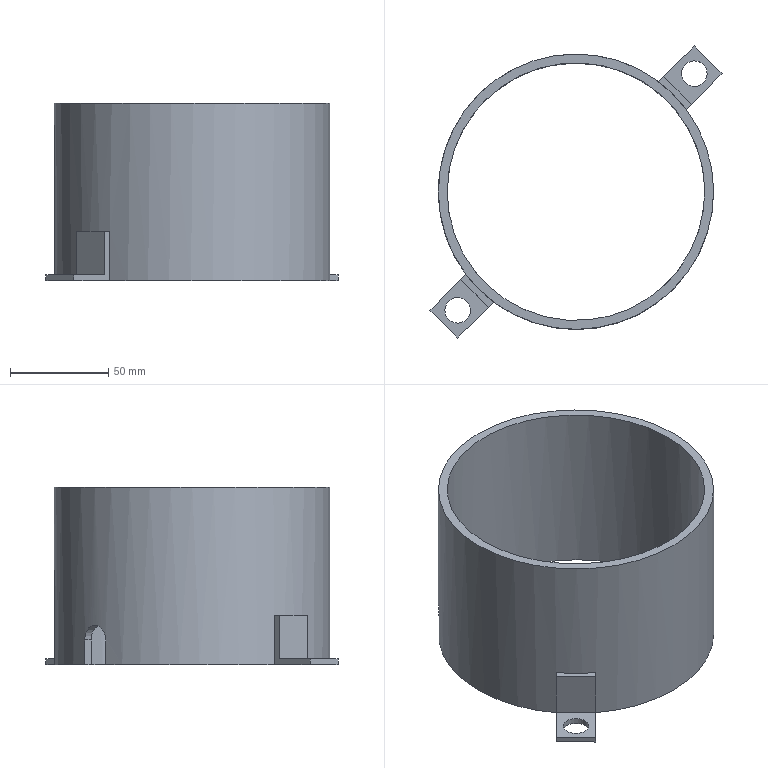Part | NX | features MAIN_BODY 2 | 1 solid | 21 faces | box 148.351 x 148.351 x 90 mm | volume 175987 mm3 | plane 16 | cylinder 5 | commonest cylinder face diameters 13 x2 15 x1 130.8 x1 139.8 x1
STEP:
#1=CARTESIAN_POINT('',(1420.523,-713.619,-12.));
#2=VERTEX_POINT('',#1);
#3=CARTESIAN_POINT('',(1420.523,-713.619,10.));
#4=VERTEX_POINT('',#3);
#5=CARTESIAN_POINT('',(1420.523,-713.619,-15.));
#6=DIRECTION('',(0.,0.,-1.));
#7=VECTOR('',#6,1000.);
#8=LINE('',#5,#7);
#9=EDGE_CURVE('',#2,#4,#8,.F.);
#10=ORIENTED_EDGE('',*,*,#9,.T.);
#11=CARTESIAN_POINT('',(1406.381,-699.477,10.));
#12=VERTEX_POINT('',#11);
#13=CARTESIAN_POINT('',(1420.523,-713.619,10.));
#14=DIRECTION('',(-0.7071,0.7071,0.));
#15=VECTOR('',#14,1000.);
#16=LINE('',#13,#15);
#17=EDGE_CURVE('',#4,#12,#16,.T.);
#18=ORIENTED_EDGE('',*,*,#17,.T.);
#19=CARTESIAN_POINT('',(1406.381,-699.477,-12.));
#20=VERTEX_POINT('',#19);
#21=CARTESIAN_POINT('',(1406.381,-699.477,-15.));
#22=DIRECTION('',(0.,0.,-1.));
#23=VECTOR('',#22,1000.);
#24=LINE('',#21,#23);
#25=EDGE_CURVE('',#20,#12,#24,.F.);
#26=ORIENTED_EDGE('',*,*,#25,.F.);
#27=CARTESIAN_POINT('',(1420.523,-713.619,-12.));
#28=DIRECTION('',(-0.7071,0.7071,0.));
#29=VECTOR('',#28,1000.);
#30=LINE('',#27,#29);
#31=EDGE_CURVE('',#2,#20,#30,.T.);
#32=ORIENTED_EDGE('',*,*,#31,.F.);
#33=EDGE_LOOP('',(#10,#18,#26,#32));
#34=FACE_BOUND('',#33,.T.);
#35=CARTESIAN_POINT('',(1420.523,-713.619,-15.));
#36=DIRECTION('',(-0.7071,-0.7071,0.));
#37=DIRECTION('',(0.,0.,-1.));
#38=AXIS2_PLACEMENT_3D('',#35,#36,#37);
#39=PLANE('',#38);
#40=ADVANCED_FACE('',(#34),#39,.T.);
#41=CARTESIAN_POINT('',(1415.573,-605.573,75.));
#42=VERTEX_POINT('',#41);
#43=CARTESIAN_POINT('',(1465.,-655.,75.));
#44=DIRECTION('',(0.,0.,-1.));
#45=DIRECTION('',(-0.7071,0.7071,0.));
#46=AXIS2_PLACEMENT_3D('',#43,#44,#45);
#47=CIRCLE('',#46,69.9);
#48=EDGE_CURVE('',#42,#42,#47,.T.);
#49=ORIENTED_EDGE('',*,*,#48,.T.);
#50=EDGE_LOOP('',(#49));
#51=FACE_BOUND('',#50,.T.);
#52=CARTESIAN_POINT('',(1423.153,-710.989,-15.));
#53=VERTEX_POINT('',#52);
#54=CARTESIAN_POINT('',(1423.153,-710.989,10.));
#55=VERTEX_POINT('',#54);
#56=CARTESIAN_POINT('',(1423.153,-710.989,75.));
#57=DIRECTION('',(0.,0.,-1.));
#58=VECTOR('',#57,1000.);
#59=LINE('',#56,#58);
#60=EDGE_CURVE('',#53,#55,#59,.F.);
#61=ORIENTED_EDGE('',*,*,#60,.F.);
#62=CARTESIAN_POINT('',(1520.989,-613.153,-15.));
#63=VERTEX_POINT('',#62);
#64=CARTESIAN_POINT('',(1465.,-655.,-15.));
#65=DIRECTION('',(0.,0.,-1.));
#66=DIRECTION('',(-0.7071,0.7071,0.));
#67=AXIS2_PLACEMENT_3D('',#64,#65,#66);
#68=CIRCLE('',#67,69.9);
#69=EDGE_CURVE('',#63,#53,#68,.T.);
#70=ORIENTED_EDGE('',*,*,#69,.F.);
#71=CARTESIAN_POINT('',(1520.989,-613.153,10.));
#72=VERTEX_POINT('',#71);
#73=CARTESIAN_POINT('',(1520.989,-613.153,75.));
#74=DIRECTION('',(0.,0.,-1.));
#75=VECTOR('',#74,1000.);
#76=LINE('',#73,#75);
#77=EDGE_CURVE('',#63,#72,#76,.F.);
#78=ORIENTED_EDGE('',*,*,#77,.T.);
#79=CARTESIAN_POINT('',(1506.847,-599.011,10.));
#80=VERTEX_POINT('',#79);
#81=CARTESIAN_POINT('',(1465.,-655.,10.));
#82=DIRECTION('',(0.,0.,1.));
#83=DIRECTION('',(0.7071,-0.7071,0.));
#84=AXIS2_PLACEMENT_3D('',#81,#82,#83);
#85=CIRCLE('',#84,69.9);
#86=EDGE_CURVE('',#72,#80,#85,.T.);
#87=ORIENTED_EDGE('',*,*,#86,.T.);
#88=CARTESIAN_POINT('',(1506.847,-599.011,-15.));
#89=VERTEX_POINT('',#88);
#90=CARTESIAN_POINT('',(1506.847,-599.011,75.));
#91=DIRECTION('',(0.,0.,-1.));
#92=VECTOR('',#91,1000.);
#93=LINE('',#90,#92);
#94=EDGE_CURVE('',#80,#89,#93,.T.);
#95=ORIENTED_EDGE('',*,*,#94,.T.);
#96=CARTESIAN_POINT('',(1421.162,-600.555,-15.));
#97=VERTEX_POINT('',#96);
#98=CARTESIAN_POINT('',(1465.,-655.,-15.));
#99=DIRECTION('',(0.,0.,-1.));
#100=DIRECTION('',(-0.7071,0.7071,0.));
#101=AXIS2_PLACEMENT_3D('',#98,#99,#100);
#102=CIRCLE('',#101,69.9);
#103=EDGE_CURVE('',#97,#89,#102,.T.);
#104=ORIENTED_EDGE('',*,*,#103,.F.);
#105=CARTESIAN_POINT('',(1421.162,-600.555,-2.5));
#106=VERTEX_POINT('',#105);
#107=CARTESIAN_POINT('',(1421.162,-600.555,75.));
#108=DIRECTION('',(0.,0.,-1.));
#109=VECTOR('',#108,1000.);
#110=LINE('',#107,#109);
#111=EDGE_CURVE('',#97,#106,#110,.F.);
#112=ORIENTED_EDGE('',*,*,#111,.T.);
#113=CARTESIAN_POINT('',(1410.555,-611.162,-2.5));
#114=VERTEX_POINT('',#113);
#115=CARTESIAN_POINT('',(1421.162,-600.555,-2.5));
#116=CARTESIAN_POINT('',(1421.162,-600.555,-0.5173));
#117=CARTESIAN_POINT('',(1419.872,-601.559,3.366));
#118=CARTESIAN_POINT('',(1415.497,-605.507,5.816));
#119=CARTESIAN_POINT('',(1411.557,-609.875,3.369));
#120=CARTESIAN_POINT('',(1410.555,-611.162,-0.5422));
#121=CARTESIAN_POINT('',(1410.555,-611.162,-2.5));
#122=B_SPLINE_CURVE_WITH_KNOTS('',3,(#115,#116,#117,#118,#119,#120,#121),.UNSPECIFIED.,.F.,.F.,(4,1,1,1,4),(0.0352,0.04107,0.04693,0.0528,0.05866),.UNSPECIFIED.);
#123=EDGE_CURVE('',#106,#114,#122,.T.);
#124=ORIENTED_EDGE('',*,*,#123,.T.);
#125=CARTESIAN_POINT('',(1410.555,-611.162,-15.));
#126=VERTEX_POINT('',#125);
#127=CARTESIAN_POINT('',(1410.555,-611.162,75.));
#128=DIRECTION('',(0.,0.,-1.));
#129=VECTOR('',#128,1000.);
#130=LINE('',#127,#129);
#131=EDGE_CURVE('',#114,#126,#130,.T.);
#132=ORIENTED_EDGE('',*,*,#131,.T.);
#133=CARTESIAN_POINT('',(1409.011,-696.847,-15.));
#134=VERTEX_POINT('',#133);
#135=CARTESIAN_POINT('',(1465.,-655.,-15.));
#136=DIRECTION('',(0.,0.,-1.));
#137=DIRECTION('',(-0.7071,0.7071,0.));
#138=AXIS2_PLACEMENT_3D('',#135,#136,#137);
#139=CIRCLE('',#138,69.9);
#140=EDGE_CURVE('',#134,#126,#139,.T.);
#141=ORIENTED_EDGE('',*,*,#140,.F.);
#142=CARTESIAN_POINT('',(1409.011,-696.847,10.));
#143=VERTEX_POINT('',#142);
#144=CARTESIAN_POINT('',(1409.011,-696.847,75.));
#145=DIRECTION('',(0.,0.,-1.));
#146=VECTOR('',#145,1000.);
#147=LINE('',#144,#146);
#148=EDGE_CURVE('',#143,#134,#147,.T.);
#149=ORIENTED_EDGE('',*,*,#148,.F.);
#150=CARTESIAN_POINT('',(1465.,-655.,10.));
#151=DIRECTION('',(0.,0.,1.));
#152=DIRECTION('',(0.7071,-0.7071,0.));
#153=AXIS2_PLACEMENT_3D('',#150,#151,#152);
#154=CIRCLE('',#153,69.9);
#155=EDGE_CURVE('',#55,#143,#154,.F.);
#156=ORIENTED_EDGE('',*,*,#155,.F.);
#157=EDGE_LOOP('',(#61,#70,#78,#87,#95,#104,#112,#124,#132,#141,#149,#156));
#158=FACE_BOUND('',#157,.T.);
#159=CARTESIAN_POINT('',(1465.,-655.,75.));
#160=DIRECTION('',(0.,0.,-1.));
#161=DIRECTION('',(0.7071,-0.7071,0.));
#162=AXIS2_PLACEMENT_3D('',#159,#160,#161);
#163=CYLINDRICAL_SURFACE('',#162,69.9);
#164=ADVANCED_FACE('',(#51,#158),#163,.T.);
#165=CARTESIAN_POINT('',(1418.755,-608.755,75.));
#166=VERTEX_POINT('',#165);
#167=CARTESIAN_POINT('',(1465.,-655.,75.));
#168=DIRECTION('',(0.,0.,-1.));
#169=DIRECTION('',(-0.7071,0.7071,0.));
#170=AXIS2_PLACEMENT_3D('',#167,#168,#169);
#171=CIRCLE('',#170,65.4);
#172=EDGE_CURVE('',#166,#166,#171,.T.);
#173=ORIENTED_EDGE('',*,*,#172,.F.);
#174=EDGE_LOOP('',(#173));
#175=FACE_BOUND('',#174,.T.);
#176=CARTESIAN_POINT('',(1424.364,-603.757,-2.5));
#177=VERTEX_POINT('',#176);
#178=CARTESIAN_POINT('',(1413.757,-614.364,-2.5));
#179=VERTEX_POINT('',#178);
#180=CARTESIAN_POINT('',(1424.364,-603.757,-2.5));
#181=CARTESIAN_POINT('',(1424.364,-603.757,-0.5167));
#182=CARTESIAN_POINT('',(1423.064,-604.75,3.366));
#183=CARTESIAN_POINT('',(1418.674,-608.685,5.816));
#184=CARTESIAN_POINT('',(1414.749,-613.067,3.369));
#185=CARTESIAN_POINT('',(1413.757,-614.364,-0.5419));
#186=CARTESIAN_POINT('',(1413.757,-614.364,-2.5));
#187=B_SPLINE_CURVE_WITH_KNOTS('',3,(#180,#181,#182,#183,#184,#185,#186),.UNSPECIFIED.,.F.,.F.,(4,1,1,1,4),(0.0352,0.04107,0.04694,0.0528,0.05867),.UNSPECIFIED.);
#188=EDGE_CURVE('',#177,#179,#187,.T.);
#189=ORIENTED_EDGE('',*,*,#188,.F.);
#190=CARTESIAN_POINT('',(1424.364,-603.757,-15.));
#191=VERTEX_POINT('',#190);
#192=CARTESIAN_POINT('',(1424.364,-603.757,75.));
#193=DIRECTION('',(0.,0.,-1.));
#194=VECTOR('',#193,1000.);
#195=LINE('',#192,#194);
#196=EDGE_CURVE('',#191,#177,#195,.F.);
#197=ORIENTED_EDGE('',*,*,#196,.F.);
#198=CARTESIAN_POINT('',(1413.757,-614.364,-15.));
#199=VERTEX_POINT('',#198);
#200=CARTESIAN_POINT('',(1465.,-655.,-15.));
#201=DIRECTION('',(0.,0.,-1.));
#202=DIRECTION('',(-0.7071,0.7071,0.));
#203=AXIS2_PLACEMENT_3D('',#200,#201,#202);
#204=CIRCLE('',#203,65.4);
#205=EDGE_CURVE('',#191,#199,#204,.T.);
#206=ORIENTED_EDGE('',*,*,#205,.T.);
#207=CARTESIAN_POINT('',(1413.757,-614.364,75.));
#208=DIRECTION('',(0.,0.,-1.));
#209=VECTOR('',#208,1000.);
#210=LINE('',#207,#209);
#211=EDGE_CURVE('',#179,#199,#210,.T.);
#212=ORIENTED_EDGE('',*,*,#211,.F.);
#213=EDGE_LOOP('',(#189,#197,#206,#212));
#214=FACE_BOUND('',#213,.T.);
#215=CARTESIAN_POINT('',(1465.,-655.,75.));
#216=DIRECTION('',(0.,0.,-1.));
#217=DIRECTION('',(0.7071,-0.7071,0.));
#218=AXIS2_PLACEMENT_3D('',#215,#216,#217);
#219=CYLINDRICAL_SURFACE('',#218,65.4);
#220=ADVANCED_FACE('',(#175,#214),#219,.F.);
#221=CARTESIAN_POINT('',(1404.967,-729.176,-15.));
#222=VERTEX_POINT('',#221);
#223=CARTESIAN_POINT('',(1390.824,-715.033,-15.));
#224=VERTEX_POINT('',#223);
#225=CARTESIAN_POINT('',(1404.967,-729.176,-15.));
#226=DIRECTION('',(-0.7071,0.7071,0.));
#227=VECTOR('',#226,1000.);
#228=LINE('',#225,#227);
#229=EDGE_CURVE('',#222,#224,#228,.T.);
#230=ORIENTED_EDGE('',*,*,#229,.T.);
#231=CARTESIAN_POINT('',(1408.502,-697.356,-15.));
#232=DIRECTION('',(-0.7071,-0.7071,0.));
#233=VECTOR('',#232,1000.);
#234=LINE('',#231,#233);
#235=EDGE_CURVE('',#134,#224,#234,.T.);
#236=ORIENTED_EDGE('',*,*,#235,.F.);
#237=ORIENTED_EDGE('',*,*,#140,.T.);
#238=CARTESIAN_POINT('',(1388.986,-589.593,-15.));
#239=DIRECTION('',(0.7071,-0.7071,0.));
#240=VECTOR('',#239,1000.);
#241=LINE('',#238,#240);
#242=EDGE_CURVE('',#126,#199,#241,.T.);
#243=ORIENTED_EDGE('',*,*,#242,.T.);
#244=ORIENTED_EDGE('',*,*,#205,.F.);
#245=CARTESIAN_POINT('',(1399.593,-578.986,-15.));
#246=DIRECTION('',(0.7071,-0.7071,0.));
#247=VECTOR('',#246,1000.);
#248=LINE('',#245,#247);
#249=EDGE_CURVE('',#97,#191,#248,.T.);
#250=ORIENTED_EDGE('',*,*,#249,.F.);
#251=ORIENTED_EDGE('',*,*,#103,.T.);
#252=CARTESIAN_POINT('',(1525.033,-580.824,-15.));
#253=VERTEX_POINT('',#252);
#254=CARTESIAN_POINT('',(1507.356,-598.502,-15.));
#255=DIRECTION('',(-0.7071,-0.7071,0.));
#256=VECTOR('',#255,1000.);
#257=LINE('',#254,#256);
#258=EDGE_CURVE('',#89,#253,#257,.F.);
#259=ORIENTED_EDGE('',*,*,#258,.T.);
#260=CARTESIAN_POINT('',(1539.176,-594.967,-15.));
#261=VERTEX_POINT('',#260);
#262=CARTESIAN_POINT('',(1539.176,-594.967,-15.));
#263=DIRECTION('',(-0.7071,0.7071,0.));
#264=VECTOR('',#263,1000.);
#265=LINE('',#262,#264);
#266=EDGE_CURVE('',#261,#253,#265,.T.);
#267=ORIENTED_EDGE('',*,*,#266,.F.);
#268=CARTESIAN_POINT('',(1521.498,-612.644,-15.));
#269=DIRECTION('',(-0.7071,-0.7071,0.));
#270=VECTOR('',#269,1000.);
#271=LINE('',#268,#270);
#272=EDGE_CURVE('',#63,#261,#271,.F.);
#273=ORIENTED_EDGE('',*,*,#272,.F.);
#274=ORIENTED_EDGE('',*,*,#69,.T.);
#275=CARTESIAN_POINT('',(1422.644,-711.498,-15.));
#276=DIRECTION('',(-0.7071,-0.7071,0.));
#277=VECTOR('',#276,1000.);
#278=LINE('',#275,#277);
#279=EDGE_CURVE('',#53,#222,#278,.T.);
#280=ORIENTED_EDGE('',*,*,#279,.T.);
#281=EDGE_LOOP('',(#230,#236,#237,#243,#244,#250,#251,#259,#267,#273,#274,#280));
#282=FACE_BOUND('',#281,.T.);
#283=CARTESIAN_POINT('',(1400.3,-710.508,-15.));
#284=VERTEX_POINT('',#283);
#285=CARTESIAN_POINT('',(1404.896,-715.104,-15.));
#286=DIRECTION('',(0.,0.,-1.));
#287=DIRECTION('',(-0.7071,0.7071,0.));
#288=AXIS2_PLACEMENT_3D('',#285,#286,#287);
#289=CIRCLE('',#288,6.5);
#290=EDGE_CURVE('',#284,#284,#289,.T.);
#291=ORIENTED_EDGE('',*,*,#290,.F.);
#292=EDGE_LOOP('',(#291));
#293=FACE_BOUND('',#292,.T.);
#294=CARTESIAN_POINT('',(1520.508,-590.3,-15.));
#295=VERTEX_POINT('',#294);
#296=CARTESIAN_POINT('',(1525.104,-594.896,-15.));
#297=DIRECTION('',(0.,0.,-1.));
#298=DIRECTION('',(-0.7071,0.7071,0.));
#299=AXIS2_PLACEMENT_3D('',#296,#297,#298);
#300=CIRCLE('',#299,6.5);
#301=EDGE_CURVE('',#295,#295,#300,.T.);
#302=ORIENTED_EDGE('',*,*,#301,.F.);
#303=EDGE_LOOP('',(#302));
#304=FACE_BOUND('',#303,.T.);
#305=CARTESIAN_POINT('',(1465.,-655.,-15.));
#306=DIRECTION('',(0.,0.,1.));
#307=DIRECTION('',(-0.7071,0.7071,0.));
#308=AXIS2_PLACEMENT_3D('',#305,#306,#307);
#309=PLANE('',#308);
#310=ADVANCED_FACE('',(#282,#293,#304),#309,.F.);
#311=ORIENTED_EDGE('',*,*,#172,.T.);
#312=EDGE_LOOP('',(#311));
#313=FACE_BOUND('',#312,.T.);
#314=ORIENTED_EDGE('',*,*,#48,.F.);
#315=EDGE_LOOP('',(#314));
#316=FACE_BOUND('',#315,.T.);
#317=CARTESIAN_POINT('',(1465.,-655.,75.));
#318=DIRECTION('',(0.,0.,1.));
#319=DIRECTION('',(-0.7071,0.7071,0.));
#320=AXIS2_PLACEMENT_3D('',#317,#318,#319);
#321=PLANE('',#320);
#322=ADVANCED_FACE('',(#313,#316),#321,.T.);
#323=CARTESIAN_POINT('',(1399.593,-578.986,-2.5));
#324=DIRECTION('',(0.7071,-0.7071,0.));
#325=VECTOR('',#324,1000.);
#326=LINE('',#323,#325);
#327=EDGE_CURVE('',#106,#177,#326,.T.);
#328=ORIENTED_EDGE('',*,*,#327,.T.);
#329=ORIENTED_EDGE('',*,*,#188,.T.);
#330=CARTESIAN_POINT('',(1388.986,-589.593,-2.5));
#331=DIRECTION('',(0.7071,-0.7071,0.));
#332=VECTOR('',#331,1000.);
#333=LINE('',#330,#332);
#334=EDGE_CURVE('',#114,#179,#333,.T.);
#335=ORIENTED_EDGE('',*,*,#334,.F.);
#336=ORIENTED_EDGE('',*,*,#123,.F.);
#337=EDGE_LOOP('',(#328,#329,#335,#336));
#338=FACE_BOUND('',#337,.T.);
#339=CARTESIAN_POINT('',(1394.289,-584.289,-2.5));
#340=DIRECTION('',(0.7071,-0.7071,0.));
#341=DIRECTION('',(0.,0.,1.));
#342=AXIS2_PLACEMENT_3D('',#339,#340,#341);
#343=CYLINDRICAL_SURFACE('',#342,7.5);
#344=ADVANCED_FACE('',(#338),#343,.F.);
#345=ORIENTED_EDGE('',*,*,#334,.T.);
#346=ORIENTED_EDGE('',*,*,#211,.T.);
#347=ORIENTED_EDGE('',*,*,#242,.F.);
#348=ORIENTED_EDGE('',*,*,#131,.F.);
#349=EDGE_LOOP('',(#345,#346,#347,#348));
#350=FACE_BOUND('',#349,.T.);
#351=CARTESIAN_POINT('',(1388.986,-589.593,-2.5));
#352=DIRECTION('',(0.7071,0.7071,0.));
#353=DIRECTION('',(0.,0.,1.));
#354=AXIS2_PLACEMENT_3D('',#351,#352,#353);
#355=PLANE('',#354);
#356=ADVANCED_FACE('',(#350),#355,.T.);
#357=ORIENTED_EDGE('',*,*,#249,.T.);
#358=ORIENTED_EDGE('',*,*,#196,.T.);
#359=ORIENTED_EDGE('',*,*,#327,.F.);
#360=ORIENTED_EDGE('',*,*,#111,.F.);
#361=EDGE_LOOP('',(#357,#358,#359,#360));
#362=FACE_BOUND('',#361,.T.);
#363=CARTESIAN_POINT('',(1399.593,-578.986,-15.));
#364=DIRECTION('',(-0.7071,-0.7071,0.));
#365=DIRECTION('',(0.,0.,-1.));
#366=AXIS2_PLACEMENT_3D('',#363,#364,#365);
#367=PLANE('',#366);
#368=ADVANCED_FACE('',(#362),#367,.T.);
#369=CARTESIAN_POINT('',(1523.619,-610.523,10.));
#370=VERTEX_POINT('',#369);
#371=CARTESIAN_POINT('',(1521.498,-612.644,10.));
#372=DIRECTION('',(-0.7071,-0.7071,0.));
#373=VECTOR('',#372,1000.);
#374=LINE('',#371,#373);
#375=EDGE_CURVE('',#72,#370,#374,.F.);
#376=ORIENTED_EDGE('',*,*,#375,.T.);
#377=CARTESIAN_POINT('',(1509.477,-596.381,10.));
#378=VERTEX_POINT('',#377);
#379=CARTESIAN_POINT('',(1523.619,-610.523,10.));
#380=DIRECTION('',(-0.7071,0.7071,0.));
#381=VECTOR('',#380,1000.);
#382=LINE('',#379,#381);
#383=EDGE_CURVE('',#370,#378,#382,.T.);
#384=ORIENTED_EDGE('',*,*,#383,.T.);
#385=CARTESIAN_POINT('',(1507.356,-598.502,10.));
#386=DIRECTION('',(-0.7071,-0.7071,0.));
#387=VECTOR('',#386,1000.);
#388=LINE('',#385,#387);
#389=EDGE_CURVE('',#80,#378,#388,.F.);
#390=ORIENTED_EDGE('',*,*,#389,.F.);
#391=ORIENTED_EDGE('',*,*,#86,.F.);
#392=EDGE_LOOP('',(#376,#384,#390,#391));
#393=FACE_BOUND('',#392,.T.);
#394=CARTESIAN_POINT('',(1521.498,-612.644,10.));
#395=DIRECTION('',(0.,0.,-1.));
#396=DIRECTION('',(-0.7071,0.7071,0.));
#397=AXIS2_PLACEMENT_3D('',#394,#395,#396);
#398=PLANE('',#397);
#399=ADVANCED_FACE('',(#393),#398,.F.);
#400=CARTESIAN_POINT('',(1525.033,-580.824,-12.));
#401=VERTEX_POINT('',#400);
#402=CARTESIAN_POINT('',(1509.477,-596.381,-12.));
#403=VERTEX_POINT('',#402);
#404=CARTESIAN_POINT('',(1507.356,-598.502,-12.));
#405=DIRECTION('',(-0.7071,-0.7071,0.));
#406=VECTOR('',#405,1000.);
#407=LINE('',#404,#406);
#408=EDGE_CURVE('',#401,#403,#407,.T.);
#409=ORIENTED_EDGE('',*,*,#408,.F.);
#410=CARTESIAN_POINT('',(1525.033,-580.824,-15.));
#411=DIRECTION('',(0.,0.,-1.));
#412=VECTOR('',#411,1000.);
#413=LINE('',#410,#412);
#414=EDGE_CURVE('',#253,#401,#413,.F.);
#415=ORIENTED_EDGE('',*,*,#414,.F.);
#416=ORIENTED_EDGE('',*,*,#258,.F.);
#417=ORIENTED_EDGE('',*,*,#94,.F.);
#418=ORIENTED_EDGE('',*,*,#389,.T.);
#419=CARTESIAN_POINT('',(1509.477,-596.381,-15.));
#420=DIRECTION('',(0.,0.,-1.));
#421=VECTOR('',#420,1000.);
#422=LINE('',#419,#421);
#423=EDGE_CURVE('',#403,#378,#422,.F.);
#424=ORIENTED_EDGE('',*,*,#423,.F.);
#425=EDGE_LOOP('',(#409,#415,#416,#417,#418,#424));
#426=FACE_BOUND('',#425,.T.);
#427=CARTESIAN_POINT('',(1507.356,-598.502,-15.));
#428=DIRECTION('',(-0.7071,0.7071,0.));
#429=DIRECTION('',(0.,0.,1.));
#430=AXIS2_PLACEMENT_3D('',#427,#428,#429);
#431=PLANE('',#430);
#432=ADVANCED_FACE('',(#426),#431,.T.);
#433=CARTESIAN_POINT('',(1523.619,-610.523,-12.));
#434=VERTEX_POINT('',#433);
#435=CARTESIAN_POINT('',(1523.619,-610.523,-15.));
#436=DIRECTION('',(0.,0.,-1.));
#437=VECTOR('',#436,1000.);
#438=LINE('',#435,#437);
#439=EDGE_CURVE('',#434,#370,#438,.F.);
#440=ORIENTED_EDGE('',*,*,#439,.T.);
#441=ORIENTED_EDGE('',*,*,#375,.F.);
#442=ORIENTED_EDGE('',*,*,#77,.F.);
#443=ORIENTED_EDGE('',*,*,#272,.T.);
#444=CARTESIAN_POINT('',(1539.176,-594.967,-12.));
#445=VERTEX_POINT('',#444);
#446=CARTESIAN_POINT('',(1539.176,-594.967,-15.));
#447=DIRECTION('',(0.,0.,-1.));
#448=VECTOR('',#447,1000.);
#449=LINE('',#446,#448);
#450=EDGE_CURVE('',#261,#445,#449,.F.);
#451=ORIENTED_EDGE('',*,*,#450,.T.);
#452=CARTESIAN_POINT('',(1521.498,-612.644,-12.));
#453=DIRECTION('',(-0.7071,-0.7071,0.));
#454=VECTOR('',#453,1000.);
#455=LINE('',#452,#454);
#456=EDGE_CURVE('',#445,#434,#455,.T.);
#457=ORIENTED_EDGE('',*,*,#456,.T.);
#458=EDGE_LOOP('',(#440,#441,#442,#443,#451,#457));
#459=FACE_BOUND('',#458,.T.);
#460=CARTESIAN_POINT('',(1521.498,-612.644,-15.));
#461=DIRECTION('',(-0.7071,0.7071,0.));
#462=DIRECTION('',(0.,0.,1.));
#463=AXIS2_PLACEMENT_3D('',#460,#461,#462);
#464=PLANE('',#463);
#465=ADVANCED_FACE('',(#459),#464,.F.);
#466=ORIENTED_EDGE('',*,*,#423,.T.);
#467=ORIENTED_EDGE('',*,*,#383,.F.);
#468=ORIENTED_EDGE('',*,*,#439,.F.);
#469=CARTESIAN_POINT('',(1523.619,-610.523,-12.));
#470=DIRECTION('',(-0.7071,0.7071,0.));
#471=VECTOR('',#470,1000.);
#472=LINE('',#469,#471);
#473=EDGE_CURVE('',#403,#434,#472,.F.);
#474=ORIENTED_EDGE('',*,*,#473,.F.);
#475=EDGE_LOOP('',(#466,#467,#468,#474));
#476=FACE_BOUND('',#475,.T.);
#477=CARTESIAN_POINT('',(1523.619,-610.523,-15.));
#478=DIRECTION('',(-0.7071,-0.7071,0.));
#479=DIRECTION('',(0.,0.,-1.));
#480=AXIS2_PLACEMENT_3D('',#477,#478,#479);
#481=PLANE('',#480);
#482=ADVANCED_FACE('',(#476),#481,.F.);
#483=CARTESIAN_POINT('',(1529.7,-599.492,-12.));
#484=VERTEX_POINT('',#483);
#485=CARTESIAN_POINT('',(1525.104,-594.896,-12.));
#486=DIRECTION('',(0.,0.,1.));
#487=DIRECTION('',(0.7071,-0.7071,0.));
#488=AXIS2_PLACEMENT_3D('',#485,#486,#487);
#489=CIRCLE('',#488,6.5);
#490=EDGE_CURVE('',#484,#484,#489,.T.);
#491=ORIENTED_EDGE('',*,*,#490,.F.);
#492=EDGE_LOOP('',(#491));
#493=FACE_BOUND('',#492,.T.);
#494=ORIENTED_EDGE('',*,*,#473,.T.);
#495=ORIENTED_EDGE('',*,*,#456,.F.);
#496=CARTESIAN_POINT('',(1539.176,-594.967,-12.));
#497=DIRECTION('',(-0.7071,0.7071,0.));
#498=VECTOR('',#497,1000.);
#499=LINE('',#496,#498);
#500=EDGE_CURVE('',#445,#401,#499,.T.);
#501=ORIENTED_EDGE('',*,*,#500,.T.);
#502=ORIENTED_EDGE('',*,*,#408,.T.);
#503=EDGE_LOOP('',(#494,#495,#501,#502));
#504=FACE_BOUND('',#503,.T.);
#505=CARTESIAN_POINT('',(1521.498,-612.644,-12.));
#506=DIRECTION('',(0.,0.,-1.));
#507=DIRECTION('',(-0.7071,0.7071,0.));
#508=AXIS2_PLACEMENT_3D('',#505,#506,#507);
#509=PLANE('',#508);
#510=ADVANCED_FACE('',(#493,#504),#509,.F.);
#511=ORIENTED_EDGE('',*,*,#500,.F.);
#512=ORIENTED_EDGE('',*,*,#450,.F.);
#513=ORIENTED_EDGE('',*,*,#266,.T.);
#514=ORIENTED_EDGE('',*,*,#414,.T.);
#515=EDGE_LOOP('',(#511,#512,#513,#514));
#516=FACE_BOUND('',#515,.T.);
#517=CARTESIAN_POINT('',(1539.176,-594.967,-15.));
#518=DIRECTION('',(-0.7071,-0.7071,0.));
#519=DIRECTION('',(0.,0.,-1.));
#520=AXIS2_PLACEMENT_3D('',#517,#518,#519);
#521=PLANE('',#520);
#522=ADVANCED_FACE('',(#516),#521,.F.);
#523=ORIENTED_EDGE('',*,*,#490,.T.);
#524=EDGE_LOOP('',(#523));
#525=FACE_BOUND('',#524,.T.);
#526=ORIENTED_EDGE('',*,*,#301,.T.);
#527=EDGE_LOOP('',(#526));
#528=FACE_BOUND('',#527,.T.);
#529=CARTESIAN_POINT('',(1525.104,-594.896,5.));
#530=DIRECTION('',(0.,0.,-1.));
#531=DIRECTION('',(0.7071,-0.7071,0.));
#532=AXIS2_PLACEMENT_3D('',#529,#530,#531);
#533=CYLINDRICAL_SURFACE('',#532,6.5);
#534=ADVANCED_FACE('',(#525,#528),#533,.F.);
#535=ORIENTED_EDGE('',*,*,#155,.T.);
#536=CARTESIAN_POINT('',(1408.502,-697.356,10.));
#537=DIRECTION('',(-0.7071,-0.7071,0.));
#538=VECTOR('',#537,1000.);
#539=LINE('',#536,#538);
#540=EDGE_CURVE('',#143,#12,#539,.T.);
#541=ORIENTED_EDGE('',*,*,#540,.T.);
#542=ORIENTED_EDGE('',*,*,#17,.F.);
#543=CARTESIAN_POINT('',(1422.644,-711.498,10.));
#544=DIRECTION('',(-0.7071,-0.7071,0.));
#545=VECTOR('',#544,1000.);
#546=LINE('',#543,#545);
#547=EDGE_CURVE('',#55,#4,#546,.T.);
#548=ORIENTED_EDGE('',*,*,#547,.F.);
#549=EDGE_LOOP('',(#535,#541,#542,#548));
#550=FACE_BOUND('',#549,.T.);
#551=CARTESIAN_POINT('',(1422.644,-711.498,10.));
#552=DIRECTION('',(0.,0.,-1.));
#553=DIRECTION('',(-0.7071,0.7071,0.));
#554=AXIS2_PLACEMENT_3D('',#551,#552,#553);
#555=PLANE('',#554);
#556=ADVANCED_FACE('',(#550),#555,.F.);
#557=ORIENTED_EDGE('',*,*,#25,.T.);
#558=ORIENTED_EDGE('',*,*,#540,.F.);
#559=ORIENTED_EDGE('',*,*,#148,.T.);
#560=ORIENTED_EDGE('',*,*,#235,.T.);
#561=CARTESIAN_POINT('',(1390.824,-715.033,-12.));
#562=VERTEX_POINT('',#561);
#563=CARTESIAN_POINT('',(1390.824,-715.033,-15.));
#564=DIRECTION('',(0.,0.,-1.));
#565=VECTOR('',#564,1000.);
#566=LINE('',#563,#565);
#567=EDGE_CURVE('',#224,#562,#566,.F.);
#568=ORIENTED_EDGE('',*,*,#567,.T.);
#569=CARTESIAN_POINT('',(1408.502,-697.356,-12.));
#570=DIRECTION('',(-0.7071,-0.7071,0.));
#571=VECTOR('',#570,1000.);
#572=LINE('',#569,#571);
#573=EDGE_CURVE('',#562,#20,#572,.F.);
#574=ORIENTED_EDGE('',*,*,#573,.T.);
#575=EDGE_LOOP('',(#557,#558,#559,#560,#568,#574));
#576=FACE_BOUND('',#575,.T.);
#577=CARTESIAN_POINT('',(1408.502,-697.356,-15.));
#578=DIRECTION('',(-0.7071,0.7071,0.));
#579=DIRECTION('',(0.,0.,1.));
#580=AXIS2_PLACEMENT_3D('',#577,#578,#579);
#581=PLANE('',#580);
#582=ADVANCED_FACE('',(#576),#581,.T.);
#583=CARTESIAN_POINT('',(1404.967,-729.176,-12.));
#584=VERTEX_POINT('',#583);
#585=CARTESIAN_POINT('',(1422.644,-711.498,-12.));
#586=DIRECTION('',(-0.7071,-0.7071,0.));
#587=VECTOR('',#586,1000.);
#588=LINE('',#585,#587);
#589=EDGE_CURVE('',#584,#2,#588,.F.);
#590=ORIENTED_EDGE('',*,*,#589,.F.);
#591=CARTESIAN_POINT('',(1404.967,-729.176,-15.));
#592=DIRECTION('',(0.,0.,-1.));
#593=VECTOR('',#592,1000.);
#594=LINE('',#591,#593);
#595=EDGE_CURVE('',#222,#584,#594,.F.);
#596=ORIENTED_EDGE('',*,*,#595,.F.);
#597=ORIENTED_EDGE('',*,*,#279,.F.);
#598=ORIENTED_EDGE('',*,*,#60,.T.);
#599=ORIENTED_EDGE('',*,*,#547,.T.);
#600=ORIENTED_EDGE('',*,*,#9,.F.);
#601=EDGE_LOOP('',(#590,#596,#597,#598,#599,#600));
#602=FACE_BOUND('',#601,.T.);
#603=CARTESIAN_POINT('',(1422.644,-711.498,-15.));
#604=DIRECTION('',(-0.7071,0.7071,0.));
#605=DIRECTION('',(0.,0.,1.));
#606=AXIS2_PLACEMENT_3D('',#603,#604,#605);
#607=PLANE('',#606);
#608=ADVANCED_FACE('',(#602),#607,.F.);
#609=ORIENTED_EDGE('',*,*,#31,.T.);
#610=ORIENTED_EDGE('',*,*,#573,.F.);
#611=CARTESIAN_POINT('',(1404.967,-729.176,-12.));
#612=DIRECTION('',(-0.7071,0.7071,0.));
#613=VECTOR('',#612,1000.);
#614=LINE('',#611,#613);
#615=EDGE_CURVE('',#584,#562,#614,.T.);
#616=ORIENTED_EDGE('',*,*,#615,.F.);
#617=ORIENTED_EDGE('',*,*,#589,.T.);
#618=EDGE_LOOP('',(#609,#610,#616,#617));
#619=FACE_BOUND('',#618,.T.);
#620=CARTESIAN_POINT('',(1409.492,-719.7,-12.));
#621=VERTEX_POINT('',#620);
#622=CARTESIAN_POINT('',(1404.896,-715.104,-12.));
#623=DIRECTION('',(0.,0.,1.));
#624=DIRECTION('',(0.7071,-0.7071,0.));
#625=AXIS2_PLACEMENT_3D('',#622,#623,#624);
#626=CIRCLE('',#625,6.5);
#627=EDGE_CURVE('',#621,#621,#626,.F.);
#628=ORIENTED_EDGE('',*,*,#627,.T.);
#629=EDGE_LOOP('',(#628));
#630=FACE_BOUND('',#629,.T.);
#631=CARTESIAN_POINT('',(1422.644,-711.498,-12.));
#632=DIRECTION('',(0.,0.,-1.));
#633=DIRECTION('',(-0.7071,0.7071,0.));
#634=AXIS2_PLACEMENT_3D('',#631,#632,#633);
#635=PLANE('',#634);
#636=ADVANCED_FACE('',(#619,#630),#635,.F.);
#637=ORIENTED_EDGE('',*,*,#615,.T.);
#638=ORIENTED_EDGE('',*,*,#567,.F.);
#639=ORIENTED_EDGE('',*,*,#229,.F.);
#640=ORIENTED_EDGE('',*,*,#595,.T.);
#641=EDGE_LOOP('',(#637,#638,#639,#640));
#642=FACE_BOUND('',#641,.T.);
#643=CARTESIAN_POINT('',(1404.967,-729.176,-15.));
#644=DIRECTION('',(-0.7071,-0.7071,0.));
#645=DIRECTION('',(0.,0.,-1.));
#646=AXIS2_PLACEMENT_3D('',#643,#644,#645);
#647=PLANE('',#646);
#648=ADVANCED_FACE('',(#642),#647,.T.);
#649=ORIENTED_EDGE('',*,*,#290,.T.);
#650=EDGE_LOOP('',(#649));
#651=FACE_BOUND('',#650,.T.);
#652=ORIENTED_EDGE('',*,*,#627,.F.);
#653=EDGE_LOOP('',(#652));
#654=FACE_BOUND('',#653,.T.);
#655=CARTESIAN_POINT('',(1404.896,-715.104,5.));
#656=DIRECTION('',(0.,0.,-1.));
#657=DIRECTION('',(0.7071,-0.7071,0.));
#658=AXIS2_PLACEMENT_3D('',#655,#656,#657);
#659=CYLINDRICAL_SURFACE('',#658,6.5);
#660=ADVANCED_FACE('',(#651,#654),#659,.F.);
#661=CLOSED_SHELL('',(#40,#164,#220,#310,#322,#344,#356,#368,#399,#432,#465,#482,#510,#522,#534,#556,#582,#608,#636,#648,#660));
#662=MANIFOLD_SOLID_BREP('',#661);
#663=(LENGTH_UNIT()NAMED_UNIT(*)SI_UNIT(.MILLI.,.METRE.));
#664=UNCERTAINTY_MEASURE_WITH_UNIT(LENGTH_MEASURE(0.0508),#663,'','');
#665=(NAMED_UNIT(*)PLANE_ANGLE_UNIT()SI_UNIT($,.RADIAN.));
#666=(NAMED_UNIT(*)SI_UNIT($,.STERADIAN.)SOLID_ANGLE_UNIT());
#667=(GEOMETRIC_REPRESENTATION_CONTEXT(3)GLOBAL_UNCERTAINTY_ASSIGNED_CONTEXT((#664))GLOBAL_UNIT_ASSIGNED_CONTEXT((#663,#665,#666))REPRESENTATION_CONTEXT('',''));
#668=ADVANCED_BREP_SHAPE_REPRESENTATION('',(#662),#667);